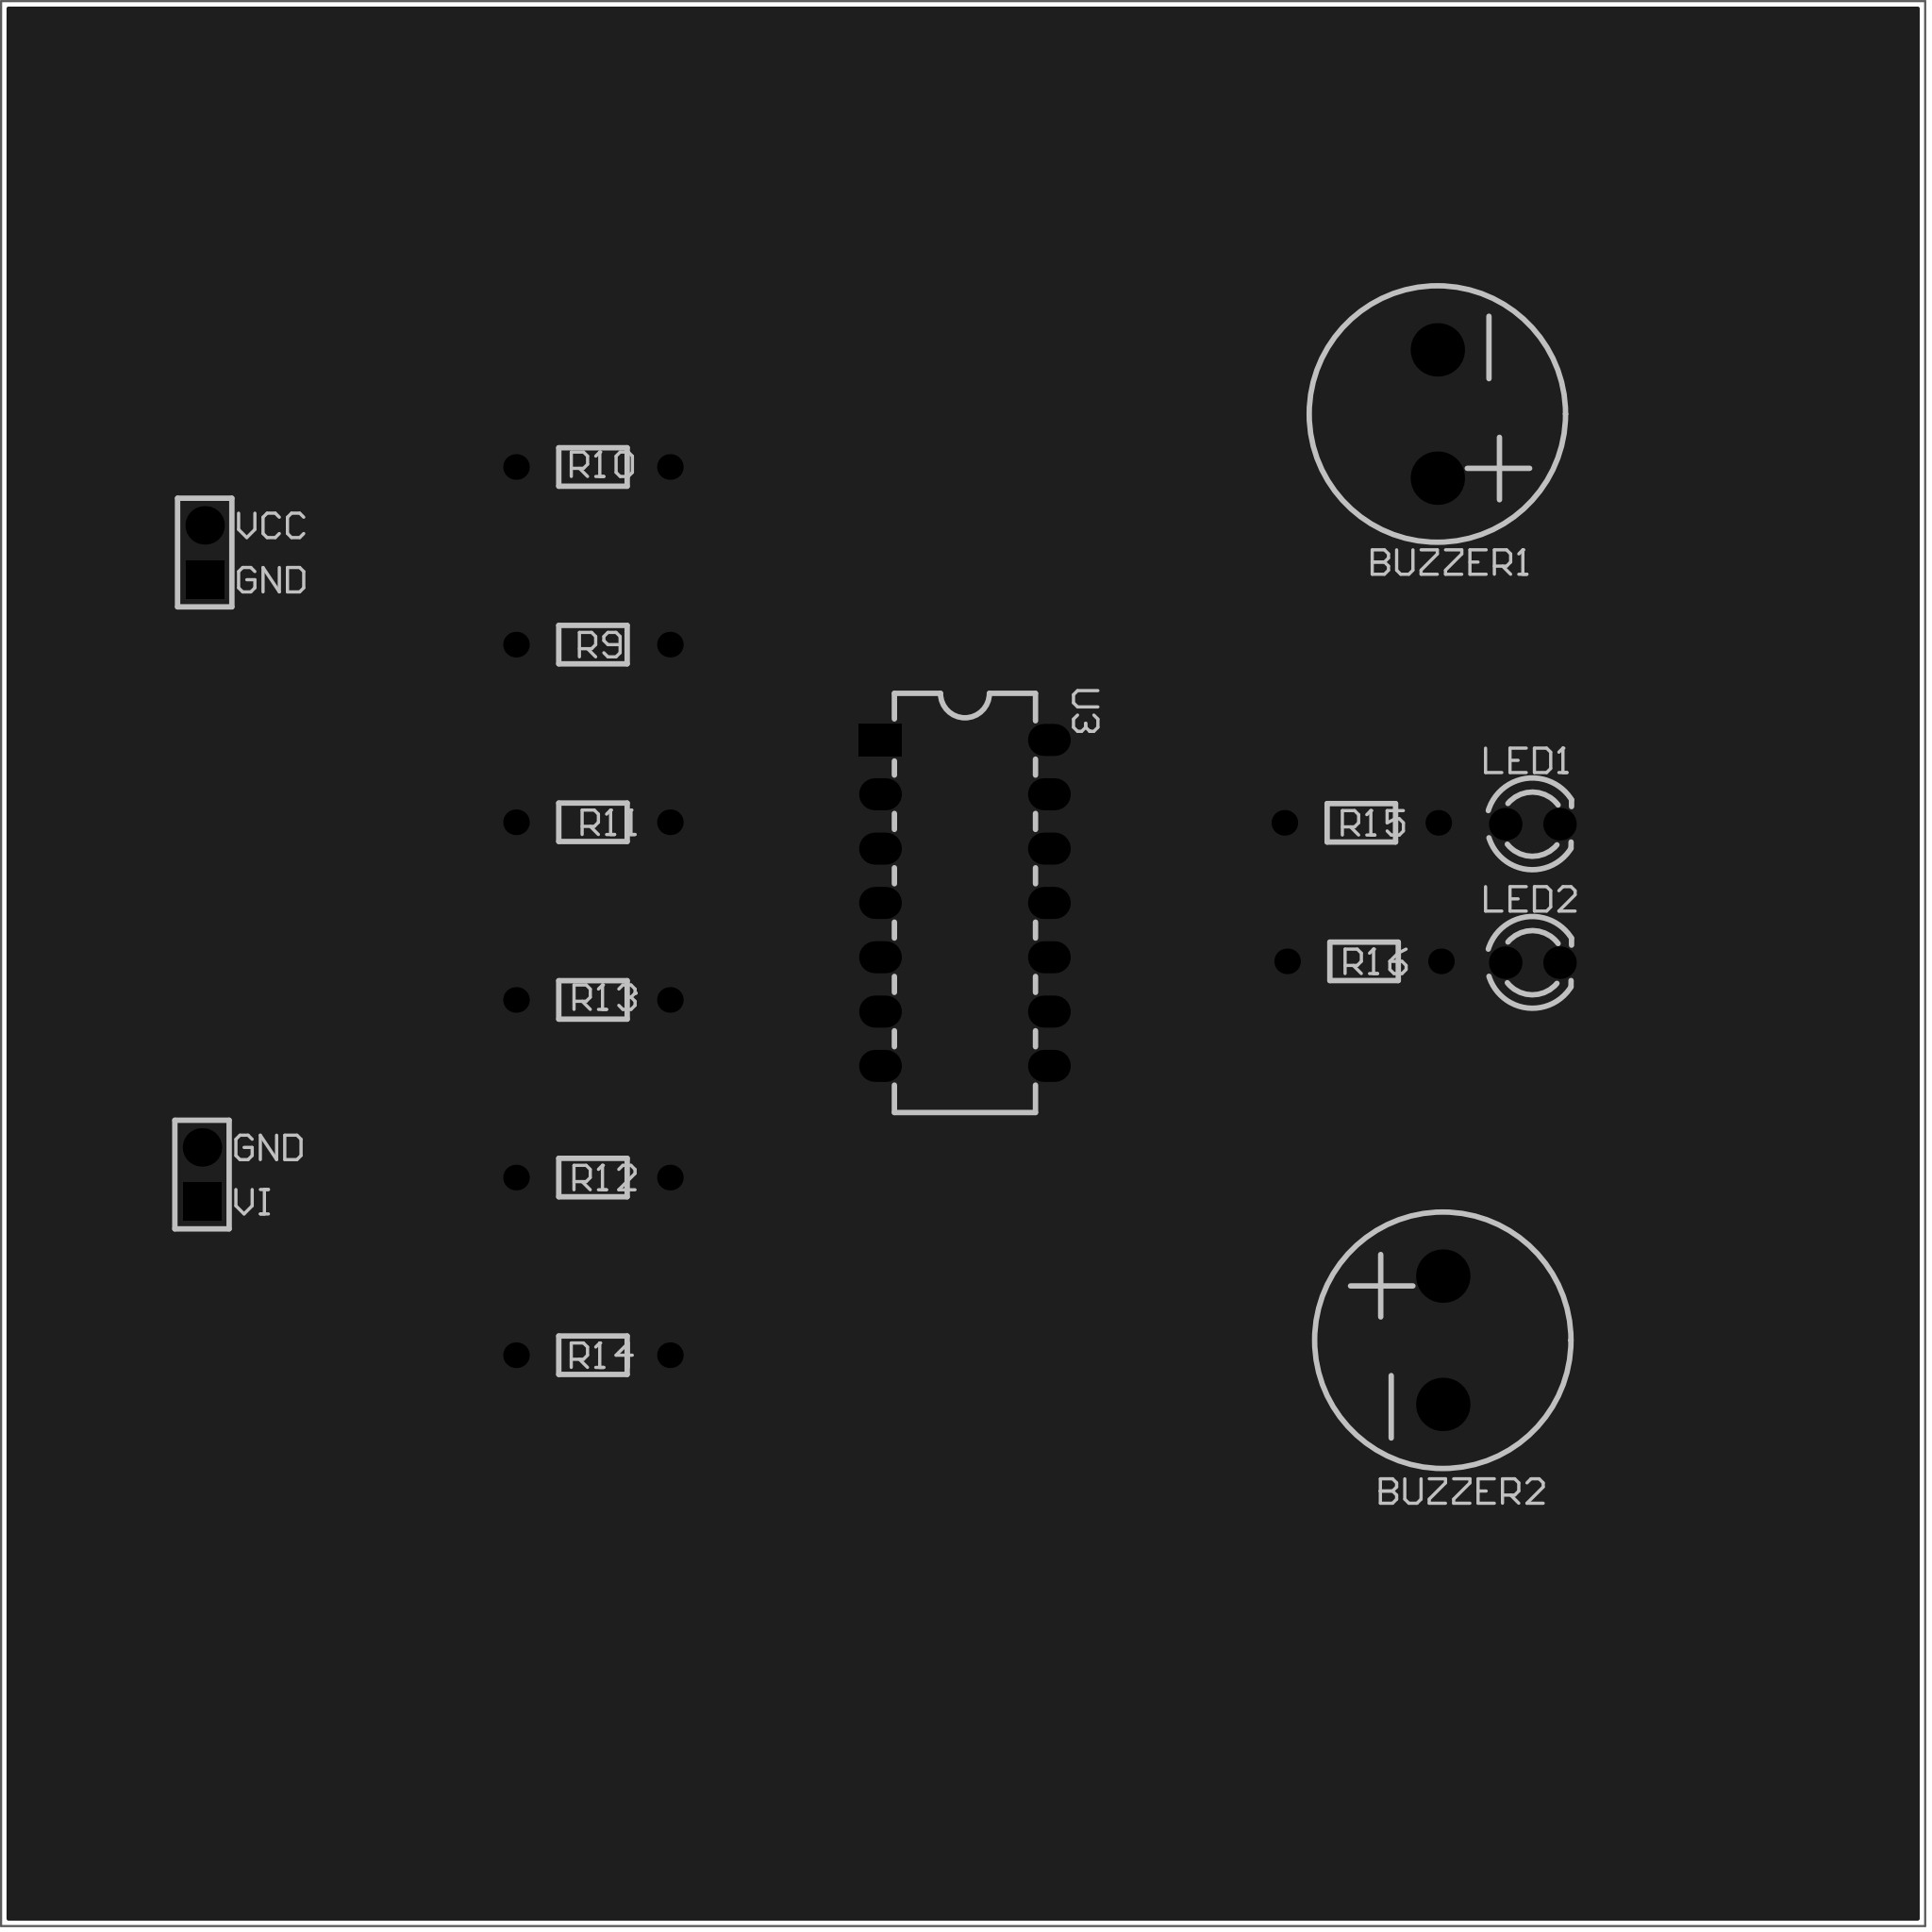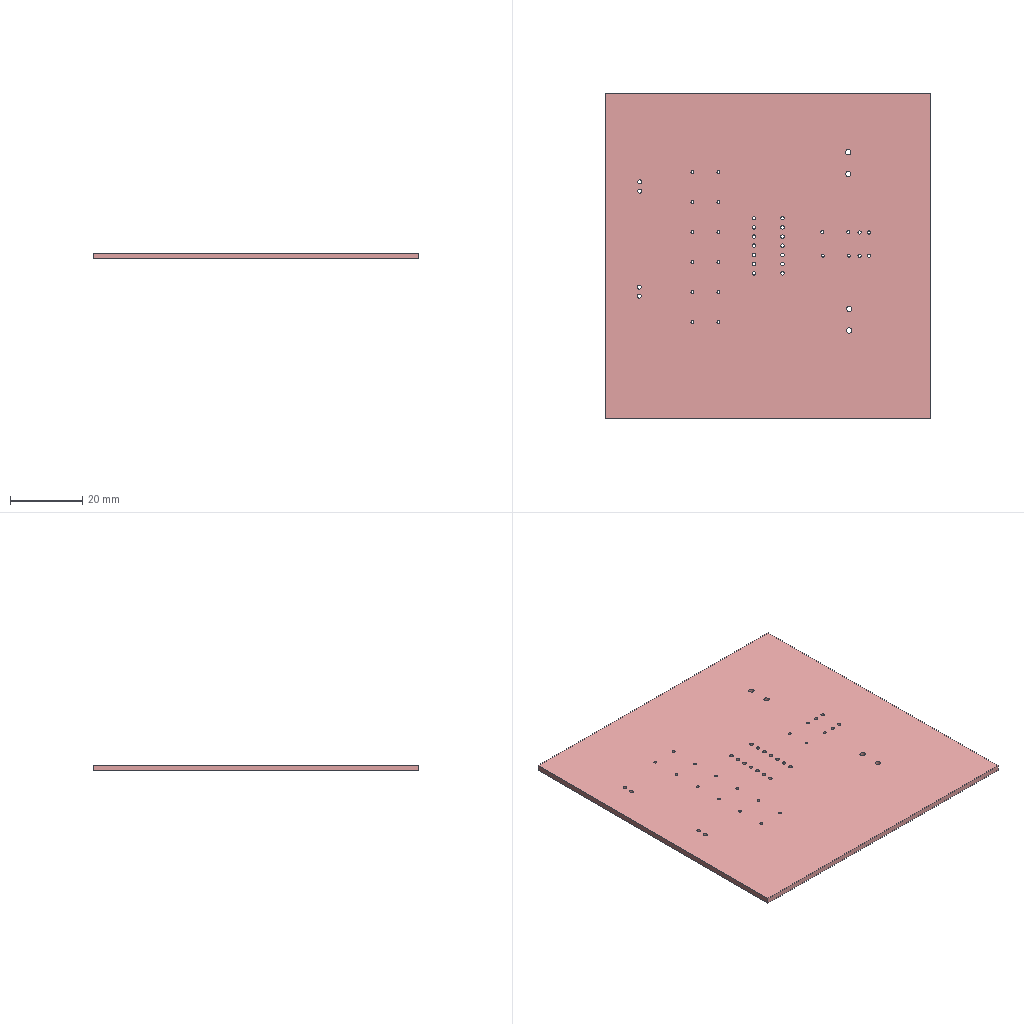Circuit board layout | Altium Designer | box 90 x 90 x 1.6 mm
Layer stack:
# Altium Designer layer stack of  (unit mm; dielectric type: 0 none, 1 core, 2 prepreg, 3 surface material)
index,name,kind,layer,copper_thickness_mm,dielectric_type,dielectric_thickness_mm,dielectric_material,dielectric_constant
0,Top Paste Mask Layer,other,,,,,,
1,Top Silkscreen Layer,other,,,,,,
2,Top Solder Mask Layer,dielectric,,,3,0.01,,3.3
3,Top Layer,copper,Top Layer,0.035,,,,
4,Dielectric1,dielectric,,,3,1.51,FR4,4.5
5,Bottom Layer,copper,Bottom Layer,0.035,,,,
6,Bottom Solder Mask Layer,dielectric,,,3,0.01,,3.3
7,Bottom Silkscreen Layer,other,,,,,,
8,Bottom Paste Mask Layer,other,,,,,,
# drill layer pairs: low layer,high layer
drill_pair,Top Layer,Bottom Layer
Part placement:
Designator,Comment,Layer,Footprint,Center-X(mm),Center-Y(mm),Rotation
H2,,TopLayer,HDR-TH_2P-P2.54-V-M-1,92.329,118.745,90
H3,,TopLayer,HDR-TH_2P-P2.54-V-M-1,92.456,147.828,90
BUZZER1,buzzer,TopLayer,BUZ-TH_BD12.0-P6.00-D0.9-RD,150.114,154.305,270
BUZZER2,buzzer,TopLayer,BUZ-TH_BD12.0-P6.00-D0.9-RD,150.368,110.998,90
U3,LM324ANE4,TopLayer,PDIP-14_L19.6-W6.5-P2.54-LS7.9-BL,128.016,131.445,270
LED1,,TopLayer,LED_TH-3mm,154.559,135.128,0
LED2,,TopLayer,LED_TH-3mm,154.559,128.651,0
R9,30K,TopLayer,Res_1/8W,110.617,143.522,0
R10,68K,TopLayer,Res_1/8W,110.617,151.828,0
R11,30K,TopLayer,Res_1/8W,110.617,135.216,180
R12,68K,TopLayer,Res_1/8W,110.617,118.605,0
R13,51K,TopLayer,Res_1/8W,110.617,126.91,0
R14,13K,TopLayer,Res_1/8W,110.617,110.299,0
R15,220,TopLayer,Res_1/8W,146.558,135.191,0
R16,220,TopLayer,Res_1/8W,146.685,128.714,0
Pad and via stacks:
# Altium Designer via and pad stacks of  (unit mm). Each distinct definition once, with the count of objects using it.
# via: kind,start_layer,end_layer,hole_mm,diameter_mm,mode(0 simple;1 top-mid-bottom;2 full stack),diameter_per_layer,count,example_net
# pad: kind,layer,hole_mm,hole_type(0 round;1 square;2 slot),plating,top_size,top_shape(1 round;2 rect;3 octagon;9 rounded rect),mid_size,bottom_size,mode,footprint,size_per_layer,count,example
pad,Multi-Layer,1.1,0,plated,1.8x1.8,1,1.8x1.8,1.8x1.8,0,HDR-TH_2P-P2.54-V-M-1,,2,H2.2
pad,Multi-Layer,1.1,0,plated,1.8x1.8,2,1.8x1.8,1.8x1.8,0,HDR-TH_2P-P2.54-V-M-1,,2,H2.1
pad,Multi-Layer,1.5,0,plated,2.5x2.5,1,2.5x2.5,2.5x2.5,0,BUZ-TH_BD12.0-P6.00-D0.9-RD,,4,BUZZER1.1
pad,Multi-Layer,1,0,plated,2x1.5,2,2x1.5,2x1.5,0,PDIP-14_L19.6-W6.5-P2.54-LS7.9-BL,,1,U3.1
pad,Multi-Layer,1,0,plated,2x1.5,1,2x1.5,2x1.5,0,PDIP-14_L19.6-W6.5-P2.54-LS7.9-BL,,13,U3.2
pad,Multi-Layer,0.9144,0,plated,1.524x1.524,1,1.524x1.524,1.524x1.524,0,LED_TH-3mm,,4,LED1.1
pad,Multi-Layer,0.8001,0,plated,1.199x1.199,1,1.199x1.199,1.199x1.199,0,Res_1/8W,,16,R9.1
Copper pours:
name,layer,net,type(0 solid;1 hatched;2 none)
Top Layer-GND,Top Layer,GND,0
Bottom Layer-GND,Bottom Layer,GND,0